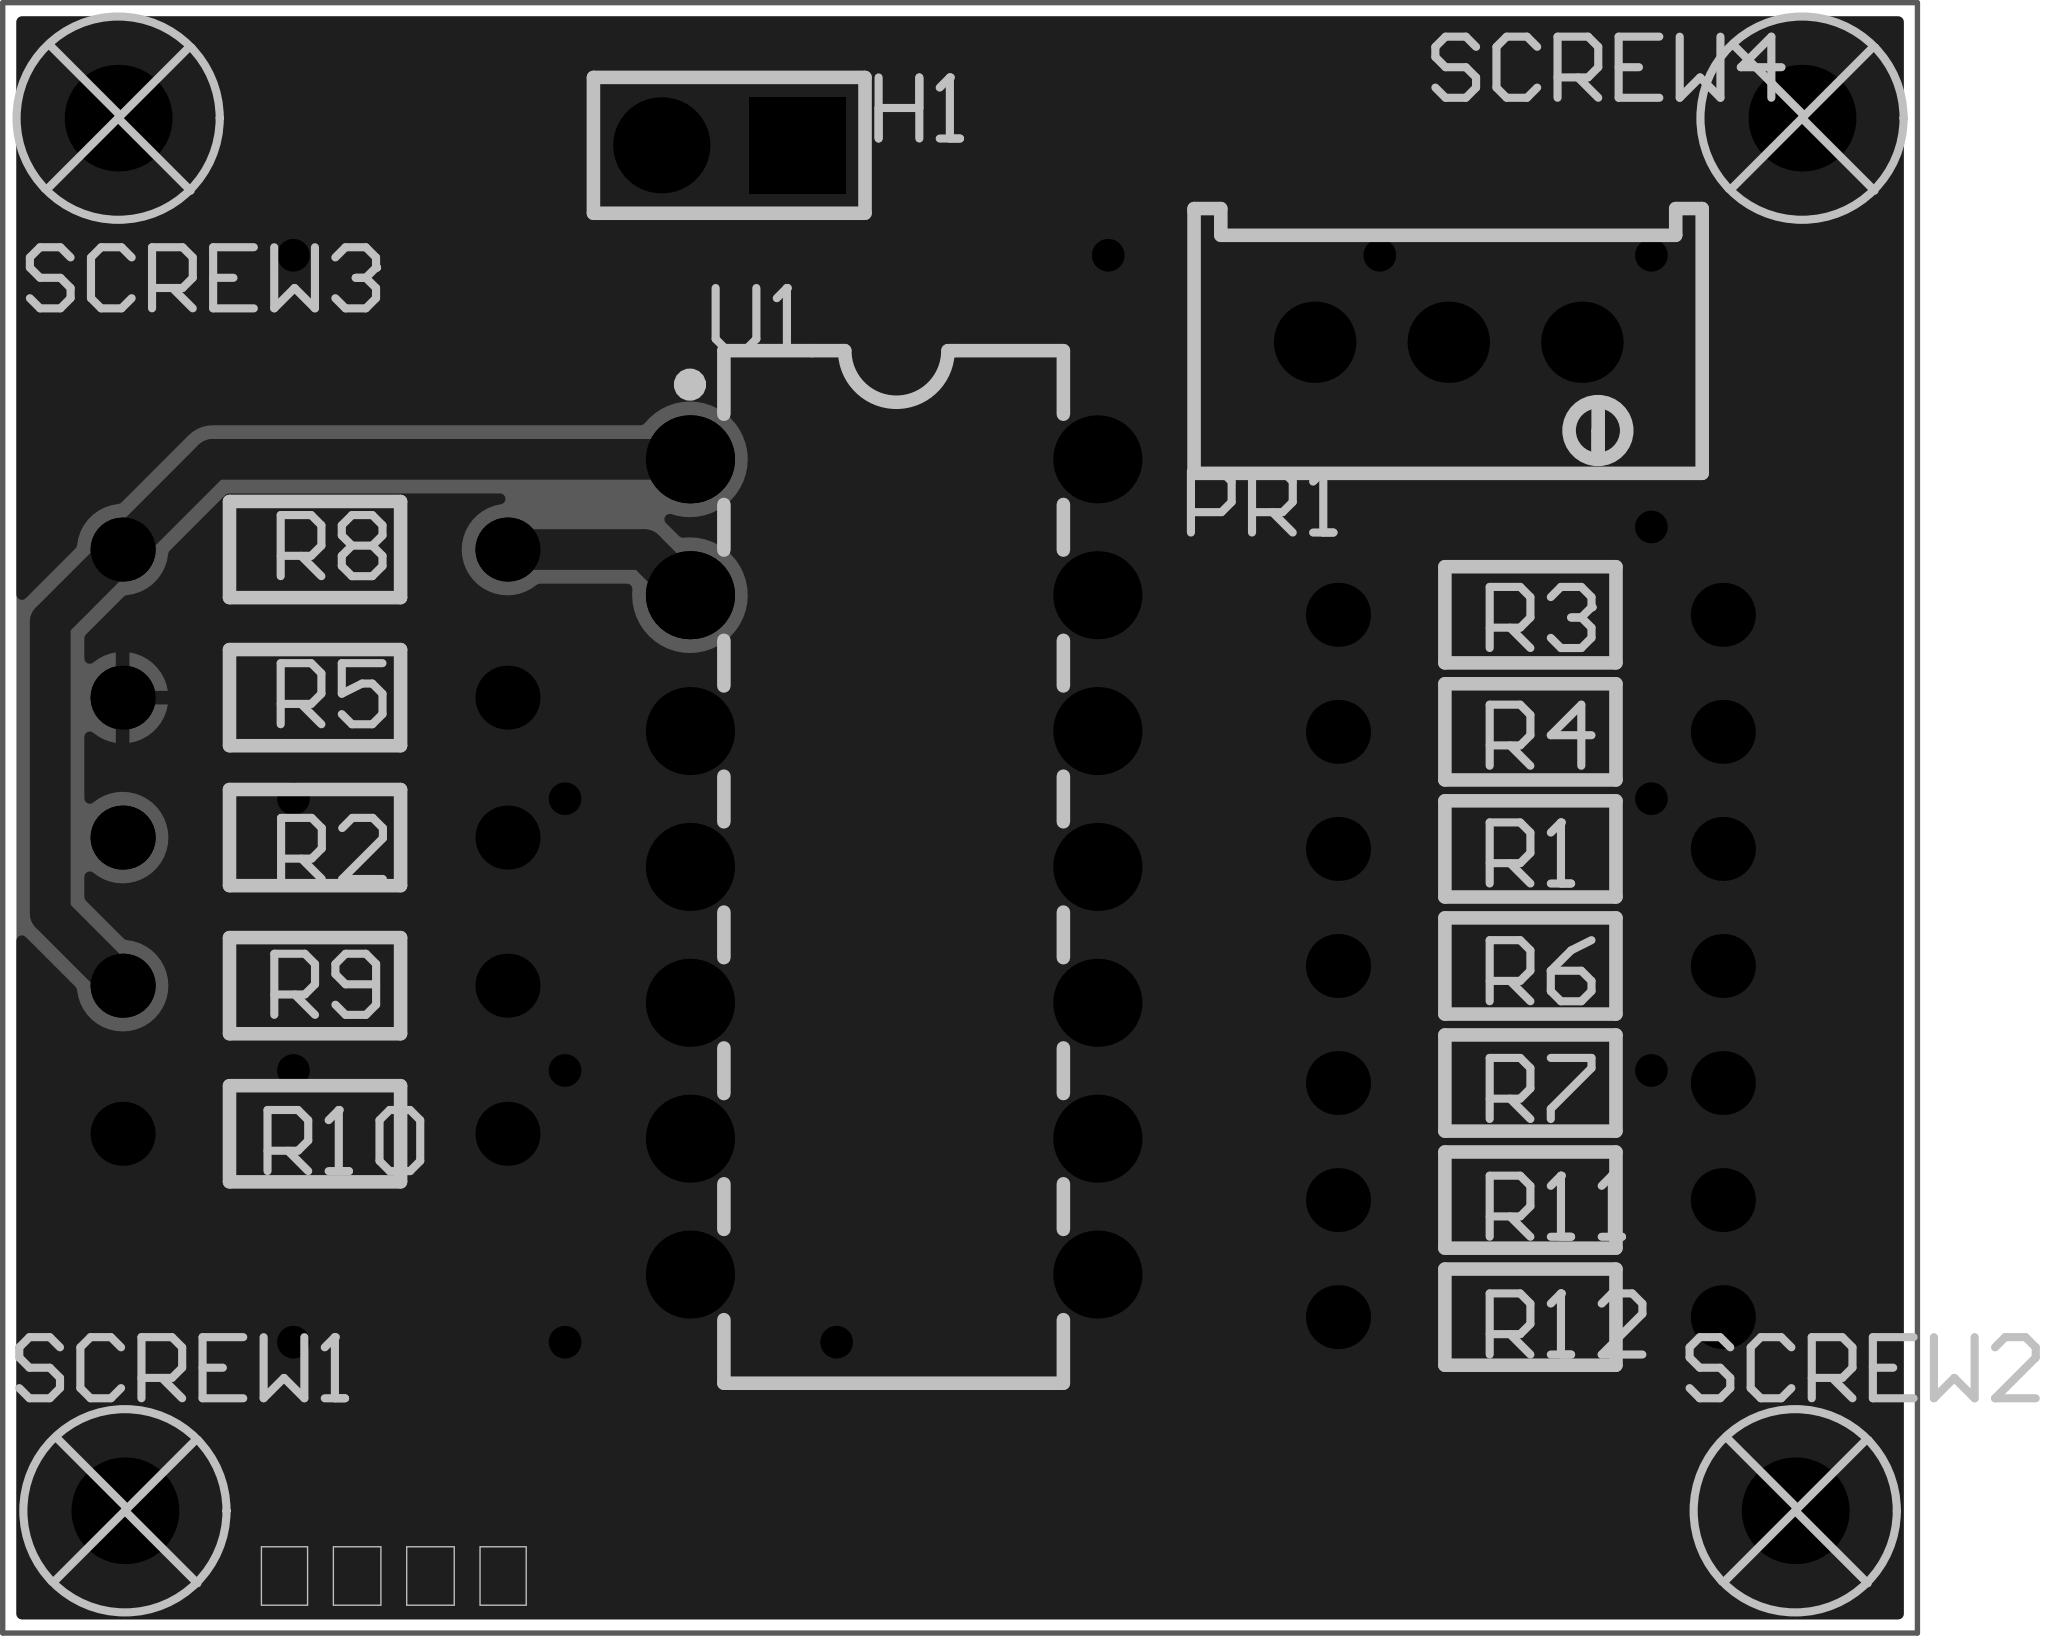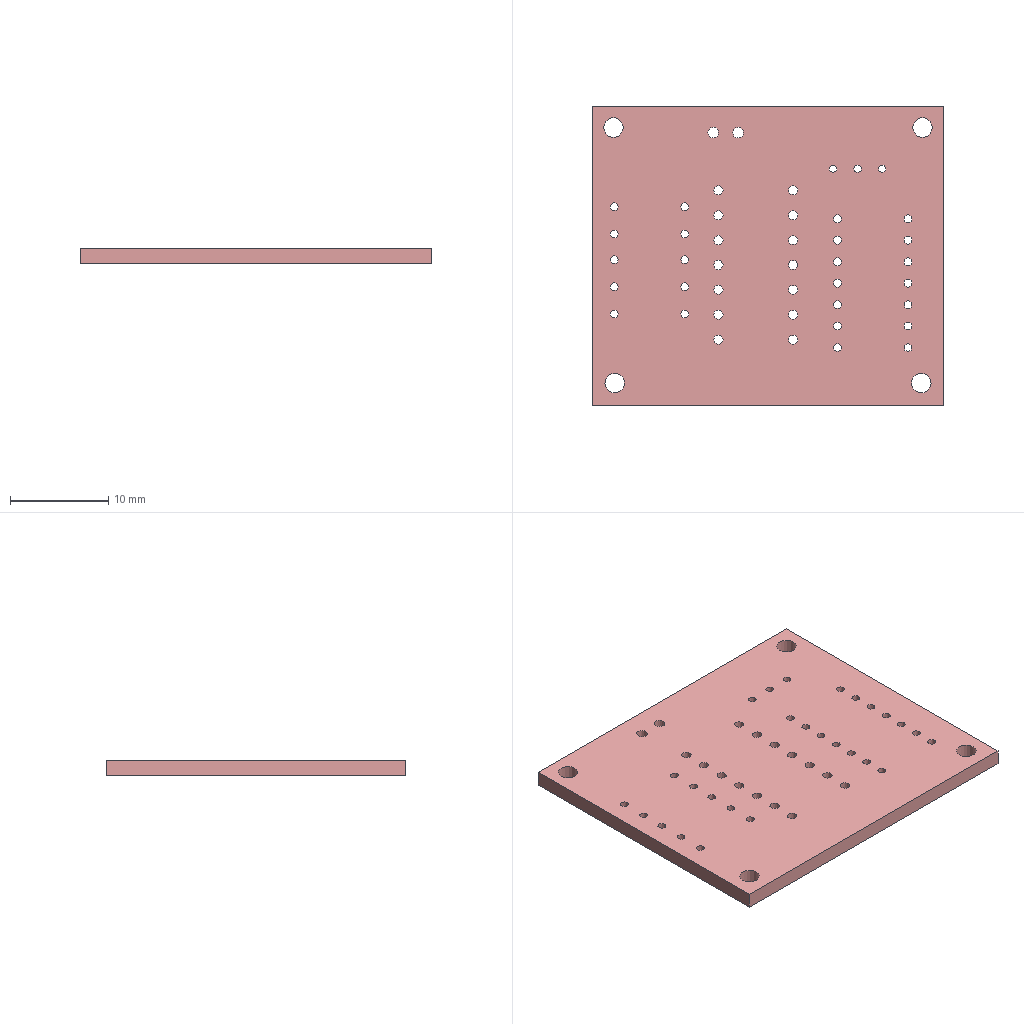Circuit board layout | Altium Designer | box 35.8 x 30.5 x 1.6 mm
Layer stack:
# Altium Designer layer stack of  (unit mm; dielectric type: 0 none, 1 core, 2 prepreg, 3 surface material)
index,name,kind,layer,copper_thickness_mm,dielectric_type,dielectric_thickness_mm,dielectric_material,dielectric_constant
0,Top Paste Mask Layer,other,,,,,,
1,Top Silkscreen Layer,other,,,,,,
2,Top Solder Mask Layer,dielectric,,,3,0.01,,3.3
3,Top Layer,copper,Top Layer,0.035,,,,
4,Dielectric1,dielectric,,,3,1.51,FR4,4.5
5,Bottom Layer,copper,Bottom Layer,0.035,,,,
6,Bottom Solder Mask Layer,dielectric,,,3,0.01,,3.3
7,Bottom Silkscreen Layer,other,,,,,,
8,Bottom Paste Mask Layer,other,,,,,,
# drill layer pairs: low layer,high layer
drill_pair,Top Layer,Bottom Layer
Part placement:
Designator,Comment,Layer,Footprint,Center-X(mm),Center-Y(mm),Rotation
PR1,10kΩ,TopLayer,R_3296,106.413,104.396,180
R1,10kΩ,TopLayer,Res_1/8W,107.95,94.923,0
R2,10kΩ,TopLayer,Res_1/8W,85.217,95.135,180
R3,9.76kΩ,TopLayer,Res_1/8W,107.95,99.3,0
R4,140Ω,TopLayer,Res_1/8W,107.95,97.112,180
R5,10kΩ,TopLayer,Res_1/8W,85.217,97.751,0
R6,2.2kΩ,TopLayer,Res_1/8W,107.95,92.735,0
R7,10kΩ,TopLayer,Res_1/8W,107.95,90.547,180
R8,10kΩ,TopLayer,Res_1/8W,85.217,100.52,0
R9,10kΩ,TopLayer,Res_1/8W,85.217,92.367,180
R10,100kΩ,TopLayer,Res_1/8W,85.217,89.598,0
R11,10kΩ,TopLayer,Res_1/8W,107.95,88.358,0
R12,100kΩ,TopLayer,Res_1/8W,107.95,86.17,180
U1,LM324N/PB,TopLayer,PDIP-14_L19.2-W6.6-P2.54-LS7.6-BL,96.039,94.587,270
SCREW1,,TopLayer,M2螺丝,81.661,82.55,0
SCREW2,,TopLayer,M2螺丝,112.903,82.55,0
SCREW3,,TopLayer,M2螺丝,81.534,108.585,0
SCREW4,,TopLayer,M2螺丝,113.03,108.585,0
H1,,TopLayer,HDR-TH_2P-P2.54-V-M-1,92.964,108.077,180
Pad and via stacks:
# Altium Designer via and pad stacks of  (unit mm). Each distinct definition once, with the count of objects using it.
# via: kind,start_layer,end_layer,hole_mm,diameter_mm,mode(0 simple;1 top-mid-bottom;2 full stack),diameter_per_layer,count,example_net
# pad: kind,layer,hole_mm,hole_type(0 round;1 square;2 slot),plating,top_size,top_shape(1 round;2 rect;3 octagon;9 rounded rect),mid_size,bottom_size,mode,footprint,size_per_layer,count,example
pad,Multi-Layer,0.762,0,plated,1.524x1.524,1,1.524x1.524,1.524x1.524,0,R_3296,,3,PR1.2
pad,Multi-Layer,0.8001,0,plated,1.199x1.199,1,1.199x1.199,1.199x1.199,0,Res_1/8W,,24,R1.1
pad,Multi-Layer,0.95,0,plated,1.65x1.65,1,1.65x1.65,1.65x1.65,0,PDIP-14_L19.2-W6.6-P2.54-LS7.6-BL,,14,U1.1
pad,Multi-Layer,2,0,plated,2x2,1,2x2,2x2,0,M2\u00C2\u00DD\u00CB\u00BF,,4,SCREW1.1
pad,Multi-Layer,1.1,0,plated,1.8x1.8,1,1.8x1.8,1.8x1.8,0,HDR-TH_2P-P2.54-V-M-1,,1,H1.2
pad,Multi-Layer,1.1,0,plated,1.8x1.8,2,1.8x1.8,1.8x1.8,0,HDR-TH_2P-P2.54-V-M-1,,1,H1.1
pad,Top Layer,0,0,plated,0.6096x0.6096,1,0.6096x0.6096,0.6096x0.6096,0,,,10,TP1
pad,Bottom Layer,0,0,plated,0.6096x0.6096,1,0.6096x0.6096,0.6096x0.6096,0,,,1,TP10
via,Top Layer,Bottom Layer,0.3048,0.61,0,,14,GND
Copper pours:
name,layer,net,type(0 solid;1 hatched;2 none)
Top Layer-GND,Top Layer,GND,0
Bottom Layer-GND,Bottom Layer,GND,0